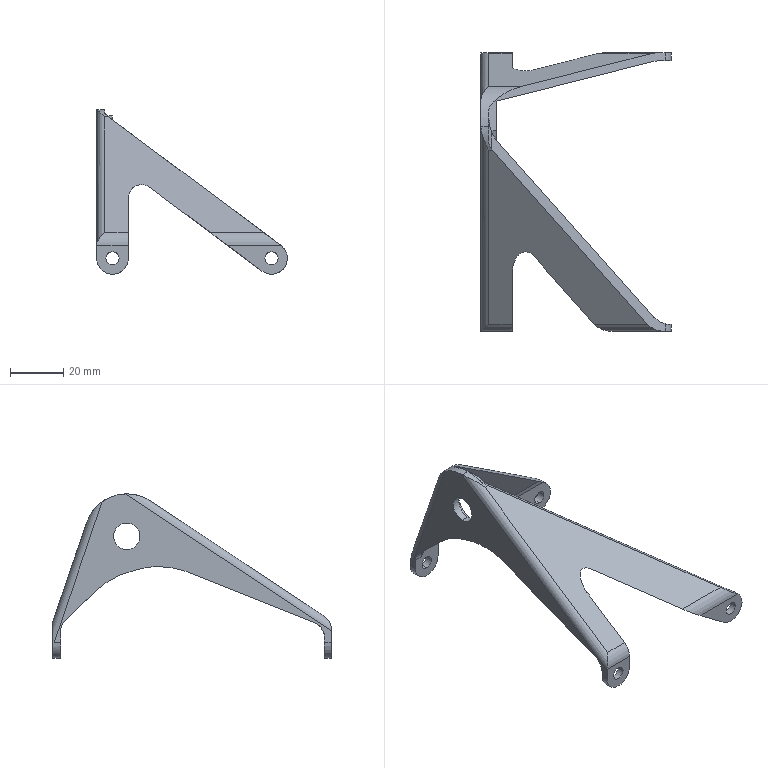Part | SolidWorks | features BaseBody 2 | 2 solids | 83 faces | box 72 x 105.202 x 62 mm | volume 17642 mm3 | cylinder 42 | plane 31 | spline 10 | commonest cylinder face diameters 12 x14 5 x8 10 x6 60 x6 6 x4 16.51 x2